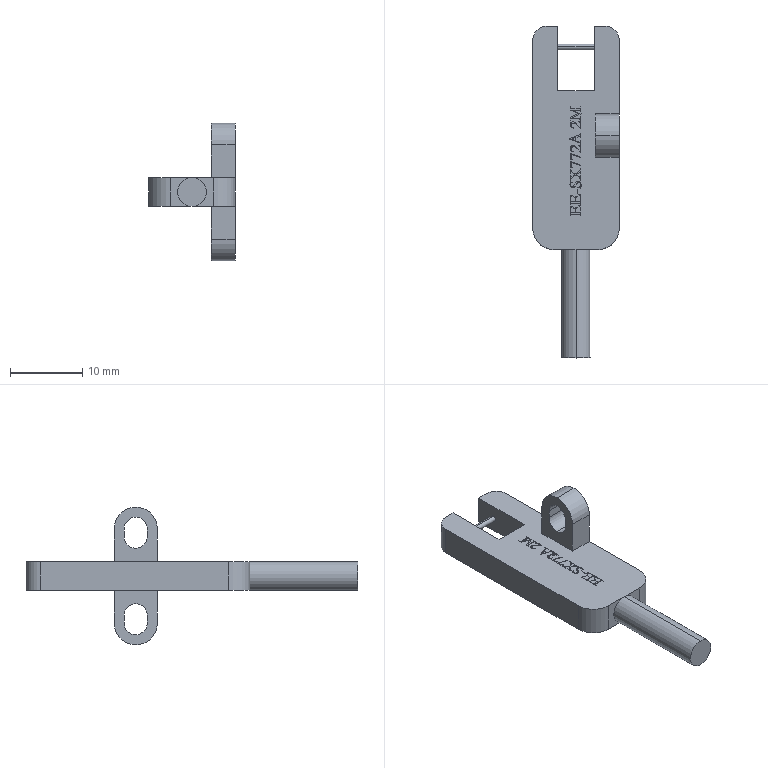Part | STEP file | QA-EE-SX772A 2M | 1 solid | 294 faces | box 12 x 46 x 19.1 mm | volume 1673 mm3 | plane 159 | spline 117 | cylinder 18 | commonest cylinder face diameters 3.2 x6 6 x6 4 x4 0.8 x2